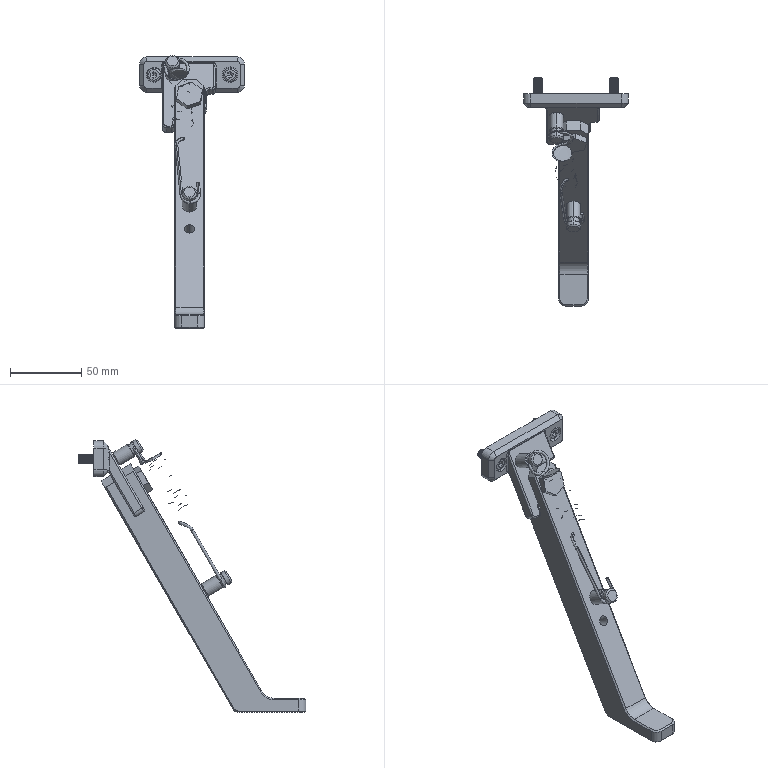Part | SolidWorks | 7 solids | 593 faces | box 73.5 x 160.086 x 191.874 mm | volume 127558 mm3 | cone 244 | cylinder 205 | plane 110 | torus 20 | spline 14 | commonest cylinder face diameters 6 x97 1.5 x28 2 x22 10 x9 8 x8 9.95 x8